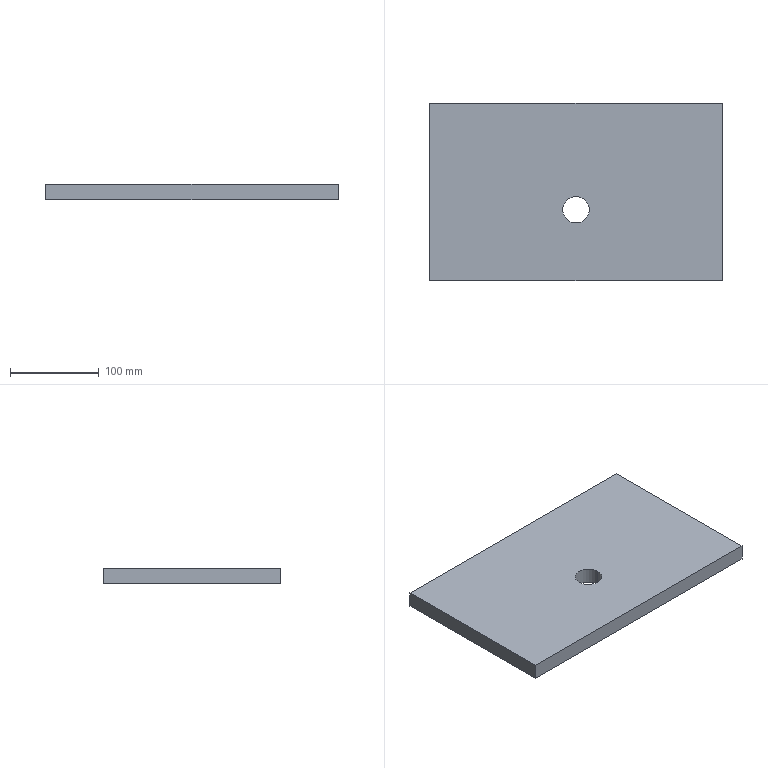Part | STEP file | PN_0031 | 1 solid | 8 faces | box 330 x 200 x 18 mm | volume 1175277 mm3 | plane 6 | cylinder 2 | commonest cylinder face diameters 30 x2
STEP:
#1=CARTESIAN_POINT('',(0.,0.,0.));
#2=DIRECTION('',(0.,0.,1.));
#3=DIRECTION('',(1.,0.,0.));
#4=AXIS2_PLACEMENT_3D('',#1,#2,#3);
#5=CARTESIAN_POINT('',(-15.,-20.,18.));
#6=VERTEX_POINT('',#5);
#7=CARTESIAN_POINT('',(-15.,-20.,0.));
#8=VERTEX_POINT('',#7);
#9=CARTESIAN_POINT('',(-15.,-20.,18.));
#10=DIRECTION('',(0.,0.,-1.));
#11=VECTOR('',#10,1.);
#12=LINE('',#9,#11);
#13=CARTESIAN_POINT('',(0.,-20.,18.));
#14=DIRECTION('',(0.,0.,-1.));
#15=DIRECTION('',(-1.,0.,0.));
#16=AXIS2_PLACEMENT_3D('',#13,#14,#15);
#17=CYLINDRICAL_SURFACE('',#16,15.);
#18=CARTESIAN_POINT('',(6.283,0.));
#19=DIRECTION('',(0.,1.));
#20=VECTOR('',#19,1.);
#21=LINE('',#18,#20);
#22=(GEOMETRIC_REPRESENTATION_CONTEXT(2)PARAMETRIC_REPRESENTATION_CONTEXT()REPRESENTATION_CONTEXT('',''));
#23=DEFINITIONAL_REPRESENTATION('',(#21),#22);
#24=PCURVE('',#17,#23);
#25=CARTESIAN_POINT('',(0.,-20.,18.));
#26=DIRECTION('',(0.,0.,-1.));
#27=DIRECTION('',(-1.,0.,0.));
#28=AXIS2_PLACEMENT_3D('',#25,#26,#27);
#29=CYLINDRICAL_SURFACE('',#28,15.);
#30=CARTESIAN_POINT('',(0.,0.));
#31=DIRECTION('',(0.,1.));
#32=VECTOR('',#31,1.);
#33=LINE('',#30,#32);
#34=(GEOMETRIC_REPRESENTATION_CONTEXT(2)PARAMETRIC_REPRESENTATION_CONTEXT()REPRESENTATION_CONTEXT('',''));
#35=DEFINITIONAL_REPRESENTATION('',(#33),#34);
#36=PCURVE('',#29,#35);
#37=SURFACE_CURVE('',#12,(#24,#36),.PCURVE_S1.);
#38=EDGE_CURVE('',#6,#8,#37,.T.);
#39=ORIENTED_EDGE('',*,*,#38,.T.);
#40=CARTESIAN_POINT('',(15.,-20.,0.));
#41=VERTEX_POINT('',#40);
#42=CARTESIAN_POINT('',(0.,-20.,0.));
#43=DIRECTION('',(0.,0.,1.));
#44=DIRECTION('',(1.,0.,0.));
#45=AXIS2_PLACEMENT_3D('',#42,#43,#44);
#46=CIRCLE('',#45,15.);
#47=CARTESIAN_POINT('',(9.425,18.));
#48=DIRECTION('',(-1.,0.));
#49=VECTOR('',#48,1.);
#50=LINE('',#47,#49);
#51=(GEOMETRIC_REPRESENTATION_CONTEXT(2)PARAMETRIC_REPRESENTATION_CONTEXT()REPRESENTATION_CONTEXT('',''));
#52=DEFINITIONAL_REPRESENTATION('',(#50),#51);
#53=PCURVE('',#17,#52);
#54=CARTESIAN_POINT('',(165.,-100.,0.));
#55=DIRECTION('',(0.,0.,1.));
#56=DIRECTION('',(1.,0.,0.));
#57=AXIS2_PLACEMENT_3D('',#54,#55,#56);
#58=PLANE('',#57);
#59=CARTESIAN_POINT('',(-165.,80.));
#60=DIRECTION('',(1.,0.));
#61=AXIS2_PLACEMENT_2D('',#59,#60);
#62=CIRCLE('',#61,15.);
#63=(GEOMETRIC_REPRESENTATION_CONTEXT(2)PARAMETRIC_REPRESENTATION_CONTEXT()REPRESENTATION_CONTEXT('',''));
#64=DEFINITIONAL_REPRESENTATION('',(#62),#63);
#65=PCURVE('',#58,#64);
#66=SURFACE_CURVE('',#46,(#53,#65),.PCURVE_S1.);
#67=EDGE_CURVE('',#8,#41,#66,.T.);
#68=ORIENTED_EDGE('',*,*,#67,.T.);
#69=CARTESIAN_POINT('',(15.,-20.,18.));
#70=VERTEX_POINT('',#69);
#71=CARTESIAN_POINT('',(15.,-20.,18.));
#72=DIRECTION('',(0.,0.,-1.));
#73=VECTOR('',#72,1.);
#74=LINE('',#71,#73);
#75=CARTESIAN_POINT('',(3.142,0.));
#76=DIRECTION('',(0.,1.));
#77=VECTOR('',#76,1.);
#78=LINE('',#75,#77);
#79=(GEOMETRIC_REPRESENTATION_CONTEXT(2)PARAMETRIC_REPRESENTATION_CONTEXT()REPRESENTATION_CONTEXT('',''));
#80=DEFINITIONAL_REPRESENTATION('',(#78),#79);
#81=PCURVE('',#17,#80);
#82=CARTESIAN_POINT('',(3.142,0.));
#83=DIRECTION('',(0.,1.));
#84=VECTOR('',#83,1.);
#85=LINE('',#82,#84);
#86=(GEOMETRIC_REPRESENTATION_CONTEXT(2)PARAMETRIC_REPRESENTATION_CONTEXT()REPRESENTATION_CONTEXT('',''));
#87=DEFINITIONAL_REPRESENTATION('',(#85),#86);
#88=PCURVE('',#29,#87);
#89=SURFACE_CURVE('',#74,(#81,#88),.PCURVE_S1.);
#90=EDGE_CURVE('',#70,#41,#89,.T.);
#91=ORIENTED_EDGE('',*,*,#90,.F.);
#92=CARTESIAN_POINT('',(0.,-20.,18.));
#93=DIRECTION('',(0.,0.,1.));
#94=DIRECTION('',(1.,0.,0.));
#95=AXIS2_PLACEMENT_3D('',#92,#93,#94);
#96=CIRCLE('',#95,15.);
#97=CARTESIAN_POINT('',(9.425,0.));
#98=DIRECTION('',(-1.,0.));
#99=VECTOR('',#98,1.);
#100=LINE('',#97,#99);
#101=(GEOMETRIC_REPRESENTATION_CONTEXT(2)PARAMETRIC_REPRESENTATION_CONTEXT()REPRESENTATION_CONTEXT('',''));
#102=DEFINITIONAL_REPRESENTATION('',(#100),#101);
#103=PCURVE('',#17,#102);
#104=CARTESIAN_POINT('',(165.,-100.,18.));
#105=DIRECTION('',(0.,0.,1.));
#106=DIRECTION('',(1.,0.,0.));
#107=AXIS2_PLACEMENT_3D('',#104,#105,#106);
#108=PLANE('',#107);
#109=CARTESIAN_POINT('',(-165.,80.));
#110=DIRECTION('',(1.,0.));
#111=AXIS2_PLACEMENT_2D('',#109,#110);
#112=CIRCLE('',#111,15.);
#113=(GEOMETRIC_REPRESENTATION_CONTEXT(2)PARAMETRIC_REPRESENTATION_CONTEXT()REPRESENTATION_CONTEXT('',''));
#114=DEFINITIONAL_REPRESENTATION('',(#112),#113);
#115=PCURVE('',#108,#114);
#116=SURFACE_CURVE('',#96,(#103,#115),.PCURVE_S1.);
#117=EDGE_CURVE('',#6,#70,#116,.T.);
#118=ORIENTED_EDGE('',*,*,#117,.F.);
#119=EDGE_LOOP('',(#39,#68,#91,#118));
#120=FACE_BOUND('',#119,.F.);
#121=ADVANCED_FACE('',(#120),#17,.F.);
#122=CARTESIAN_POINT('',(165.,-100.,18.));
#123=VERTEX_POINT('',#122);
#124=CARTESIAN_POINT('',(165.,100.,18.));
#125=VERTEX_POINT('',#124);
#126=CARTESIAN_POINT('',(165.,100.,18.));
#127=DIRECTION('',(0.,1.,0.));
#128=VECTOR('',#127,1.);
#129=LINE('',#126,#128);
#130=CARTESIAN_POINT('',(0.,200.));
#131=DIRECTION('',(0.,1.));
#132=VECTOR('',#131,1.);
#133=LINE('',#130,#132);
#134=(GEOMETRIC_REPRESENTATION_CONTEXT(2)PARAMETRIC_REPRESENTATION_CONTEXT()REPRESENTATION_CONTEXT('',''));
#135=DEFINITIONAL_REPRESENTATION('',(#133),#134);
#136=PCURVE('',#108,#135);
#137=CARTESIAN_POINT('',(165.,100.,18.));
#138=DIRECTION('',(-1.,0.,0.));
#139=DIRECTION('',(0.,0.,1.));
#140=AXIS2_PLACEMENT_3D('',#137,#138,#139);
#141=PLANE('',#140);
#142=CARTESIAN_POINT('',(0.,0.));
#143=DIRECTION('',(0.,1.));
#144=VECTOR('',#143,1.);
#145=LINE('',#142,#144);
#146=(GEOMETRIC_REPRESENTATION_CONTEXT(2)PARAMETRIC_REPRESENTATION_CONTEXT()REPRESENTATION_CONTEXT('',''));
#147=DEFINITIONAL_REPRESENTATION('',(#145),#146);
#148=PCURVE('',#141,#147);
#149=SURFACE_CURVE('',#129,(#136,#148),.PCURVE_S1.);
#150=EDGE_CURVE('',#123,#125,#149,.T.);
#151=ORIENTED_EDGE('',*,*,#150,.T.);
#152=CARTESIAN_POINT('',(-165.,100.,18.));
#153=VERTEX_POINT('',#152);
#154=CARTESIAN_POINT('',(-165.,100.,18.));
#155=DIRECTION('',(-1.,0.,0.));
#156=VECTOR('',#155,1.);
#157=LINE('',#154,#156);
#158=CARTESIAN_POINT('',(-330.,200.));
#159=DIRECTION('',(-1.,0.));
#160=VECTOR('',#159,1.);
#161=LINE('',#158,#160);
#162=(GEOMETRIC_REPRESENTATION_CONTEXT(2)PARAMETRIC_REPRESENTATION_CONTEXT()REPRESENTATION_CONTEXT('',''));
#163=DEFINITIONAL_REPRESENTATION('',(#161),#162);
#164=PCURVE('',#108,#163);
#165=CARTESIAN_POINT('',(-165.,100.,18.));
#166=DIRECTION('',(0.,-1.,0.));
#167=DIRECTION('',(0.,0.,-1.));
#168=AXIS2_PLACEMENT_3D('',#165,#166,#167);
#169=PLANE('',#168);
#170=CARTESIAN_POINT('',(0.,0.));
#171=DIRECTION('',(0.,-1.));
#172=VECTOR('',#171,1.);
#173=LINE('',#170,#172);
#174=(GEOMETRIC_REPRESENTATION_CONTEXT(2)PARAMETRIC_REPRESENTATION_CONTEXT()REPRESENTATION_CONTEXT('',''));
#175=DEFINITIONAL_REPRESENTATION('',(#173),#174);
#176=PCURVE('',#169,#175);
#177=SURFACE_CURVE('',#157,(#164,#176),.PCURVE_S1.);
#178=EDGE_CURVE('',#125,#153,#177,.T.);
#179=ORIENTED_EDGE('',*,*,#178,.T.);
#180=CARTESIAN_POINT('',(-165.,-100.,18.));
#181=VERTEX_POINT('',#180);
#182=CARTESIAN_POINT('',(-165.,100.,18.));
#183=DIRECTION('',(0.,-1.,0.));
#184=VECTOR('',#183,1.);
#185=LINE('',#182,#184);
#186=CARTESIAN_POINT('',(-330.,200.));
#187=DIRECTION('',(0.,-1.));
#188=VECTOR('',#187,1.);
#189=LINE('',#186,#188);
#190=(GEOMETRIC_REPRESENTATION_CONTEXT(2)PARAMETRIC_REPRESENTATION_CONTEXT()REPRESENTATION_CONTEXT('',''));
#191=DEFINITIONAL_REPRESENTATION('',(#189),#190);
#192=PCURVE('',#108,#191);
#193=CARTESIAN_POINT('',(-165.,100.,18.));
#194=DIRECTION('',(1.,0.,0.));
#195=DIRECTION('',(0.,1.,0.));
#196=AXIS2_PLACEMENT_3D('',#193,#194,#195);
#197=PLANE('',#196);
#198=CARTESIAN_POINT('',(0.,0.));
#199=DIRECTION('',(-1.,0.));
#200=VECTOR('',#199,1.);
#201=LINE('',#198,#200);
#202=(GEOMETRIC_REPRESENTATION_CONTEXT(2)PARAMETRIC_REPRESENTATION_CONTEXT()REPRESENTATION_CONTEXT('',''));
#203=DEFINITIONAL_REPRESENTATION('',(#201),#202);
#204=PCURVE('',#197,#203);
#205=SURFACE_CURVE('',#185,(#192,#204),.PCURVE_S1.);
#206=EDGE_CURVE('',#153,#181,#205,.T.);
#207=ORIENTED_EDGE('',*,*,#206,.T.);
#208=CARTESIAN_POINT('',(-165.,-100.,18.));
#209=DIRECTION('',(1.,0.,0.));
#210=VECTOR('',#209,1.);
#211=LINE('',#208,#210);
#212=CARTESIAN_POINT('',(-330.,0.));
#213=DIRECTION('',(1.,0.));
#214=VECTOR('',#213,1.);
#215=LINE('',#212,#214);
#216=(GEOMETRIC_REPRESENTATION_CONTEXT(2)PARAMETRIC_REPRESENTATION_CONTEXT()REPRESENTATION_CONTEXT('',''));
#217=DEFINITIONAL_REPRESENTATION('',(#215),#216);
#218=PCURVE('',#108,#217);
#219=CARTESIAN_POINT('',(-165.,-100.,18.));
#220=DIRECTION('',(0.,1.,0.));
#221=DIRECTION('',(-1.,0.,0.));
#222=AXIS2_PLACEMENT_3D('',#219,#220,#221);
#223=PLANE('',#222);
#224=CARTESIAN_POINT('',(0.,0.));
#225=DIRECTION('',(-1.,0.));
#226=VECTOR('',#225,1.);
#227=LINE('',#224,#226);
#228=(GEOMETRIC_REPRESENTATION_CONTEXT(2)PARAMETRIC_REPRESENTATION_CONTEXT()REPRESENTATION_CONTEXT('',''));
#229=DEFINITIONAL_REPRESENTATION('',(#227),#228);
#230=PCURVE('',#223,#229);
#231=SURFACE_CURVE('',#211,(#218,#230),.PCURVE_S1.);
#232=EDGE_CURVE('',#181,#123,#231,.T.);
#233=ORIENTED_EDGE('',*,*,#232,.T.);
#234=EDGE_LOOP('',(#151,#179,#207,#233));
#235=FACE_BOUND('',#234,.T.);
#236=ORIENTED_EDGE('',*,*,#117,.F.);
#237=CARTESIAN_POINT('',(0.,-20.,18.));
#238=DIRECTION('',(0.,0.,1.));
#239=DIRECTION('',(1.,0.,0.));
#240=AXIS2_PLACEMENT_3D('',#237,#238,#239);
#241=CIRCLE('',#240,15.);
#242=CARTESIAN_POINT('',(-165.,80.));
#243=DIRECTION('',(1.,0.));
#244=AXIS2_PLACEMENT_2D('',#242,#243);
#245=CIRCLE('',#244,15.);
#246=(GEOMETRIC_REPRESENTATION_CONTEXT(2)PARAMETRIC_REPRESENTATION_CONTEXT()REPRESENTATION_CONTEXT('',''));
#247=DEFINITIONAL_REPRESENTATION('',(#245),#246);
#248=PCURVE('',#108,#247);
#249=CARTESIAN_POINT('',(3.142,0.));
#250=DIRECTION('',(-1.,0.));
#251=VECTOR('',#250,1.);
#252=LINE('',#249,#251);
#253=(GEOMETRIC_REPRESENTATION_CONTEXT(2)PARAMETRIC_REPRESENTATION_CONTEXT()REPRESENTATION_CONTEXT('',''));
#254=DEFINITIONAL_REPRESENTATION('',(#252),#253);
#255=PCURVE('',#29,#254);
#256=SURFACE_CURVE('',#241,(#248,#255),.PCURVE_S1.);
#257=EDGE_CURVE('',#70,#6,#256,.T.);
#258=ORIENTED_EDGE('',*,*,#257,.F.);
#259=EDGE_LOOP('',(#236,#258));
#260=FACE_BOUND('',#259,.T.);
#261=ADVANCED_FACE('',(#235,#260),#108,.T.);
#262=CARTESIAN_POINT('',(165.,-100.,0.));
#263=VERTEX_POINT('',#262);
#264=CARTESIAN_POINT('',(165.,100.,0.));
#265=VERTEX_POINT('',#264);
#266=CARTESIAN_POINT('',(165.,100.,0.));
#267=DIRECTION('',(0.,1.,0.));
#268=VECTOR('',#267,1.);
#269=LINE('',#266,#268);
#270=CARTESIAN_POINT('',(0.,200.));
#271=DIRECTION('',(0.,1.));
#272=VECTOR('',#271,1.);
#273=LINE('',#270,#272);
#274=(GEOMETRIC_REPRESENTATION_CONTEXT(2)PARAMETRIC_REPRESENTATION_CONTEXT()REPRESENTATION_CONTEXT('',''));
#275=DEFINITIONAL_REPRESENTATION('',(#273),#274);
#276=PCURVE('',#58,#275);
#277=CARTESIAN_POINT('',(-18.,0.));
#278=DIRECTION('',(0.,1.));
#279=VECTOR('',#278,1.);
#280=LINE('',#277,#279);
#281=(GEOMETRIC_REPRESENTATION_CONTEXT(2)PARAMETRIC_REPRESENTATION_CONTEXT()REPRESENTATION_CONTEXT('',''));
#282=DEFINITIONAL_REPRESENTATION('',(#280),#281);
#283=PCURVE('',#141,#282);
#284=SURFACE_CURVE('',#269,(#276,#283),.PCURVE_S1.);
#285=EDGE_CURVE('',#263,#265,#284,.T.);
#286=ORIENTED_EDGE('',*,*,#285,.F.);
#287=CARTESIAN_POINT('',(-165.,-100.,0.));
#288=VERTEX_POINT('',#287);
#289=CARTESIAN_POINT('',(-165.,-100.,0.));
#290=DIRECTION('',(1.,0.,0.));
#291=VECTOR('',#290,1.);
#292=LINE('',#289,#291);
#293=CARTESIAN_POINT('',(-330.,0.));
#294=DIRECTION('',(1.,0.));
#295=VECTOR('',#294,1.);
#296=LINE('',#293,#295);
#297=(GEOMETRIC_REPRESENTATION_CONTEXT(2)PARAMETRIC_REPRESENTATION_CONTEXT()REPRESENTATION_CONTEXT('',''));
#298=DEFINITIONAL_REPRESENTATION('',(#296),#297);
#299=PCURVE('',#58,#298);
#300=CARTESIAN_POINT('',(0.,-18.));
#301=DIRECTION('',(-1.,0.));
#302=VECTOR('',#301,1.);
#303=LINE('',#300,#302);
#304=(GEOMETRIC_REPRESENTATION_CONTEXT(2)PARAMETRIC_REPRESENTATION_CONTEXT()REPRESENTATION_CONTEXT('',''));
#305=DEFINITIONAL_REPRESENTATION('',(#303),#304);
#306=PCURVE('',#223,#305);
#307=SURFACE_CURVE('',#292,(#299,#306),.PCURVE_S1.);
#308=EDGE_CURVE('',#288,#263,#307,.T.);
#309=ORIENTED_EDGE('',*,*,#308,.F.);
#310=CARTESIAN_POINT('',(-165.,100.,0.));
#311=VERTEX_POINT('',#310);
#312=CARTESIAN_POINT('',(-165.,100.,0.));
#313=DIRECTION('',(0.,-1.,0.));
#314=VECTOR('',#313,1.);
#315=LINE('',#312,#314);
#316=CARTESIAN_POINT('',(-330.,200.));
#317=DIRECTION('',(0.,-1.));
#318=VECTOR('',#317,1.);
#319=LINE('',#316,#318);
#320=(GEOMETRIC_REPRESENTATION_CONTEXT(2)PARAMETRIC_REPRESENTATION_CONTEXT()REPRESENTATION_CONTEXT('',''));
#321=DEFINITIONAL_REPRESENTATION('',(#319),#320);
#322=PCURVE('',#58,#321);
#323=CARTESIAN_POINT('',(0.,-18.));
#324=DIRECTION('',(-1.,0.));
#325=VECTOR('',#324,1.);
#326=LINE('',#323,#325);
#327=(GEOMETRIC_REPRESENTATION_CONTEXT(2)PARAMETRIC_REPRESENTATION_CONTEXT()REPRESENTATION_CONTEXT('',''));
#328=DEFINITIONAL_REPRESENTATION('',(#326),#327);
#329=PCURVE('',#197,#328);
#330=SURFACE_CURVE('',#315,(#322,#329),.PCURVE_S1.);
#331=EDGE_CURVE('',#311,#288,#330,.T.);
#332=ORIENTED_EDGE('',*,*,#331,.F.);
#333=CARTESIAN_POINT('',(-165.,100.,0.));
#334=DIRECTION('',(-1.,0.,0.));
#335=VECTOR('',#334,1.);
#336=LINE('',#333,#335);
#337=CARTESIAN_POINT('',(-330.,200.));
#338=DIRECTION('',(-1.,0.));
#339=VECTOR('',#338,1.);
#340=LINE('',#337,#339);
#341=(GEOMETRIC_REPRESENTATION_CONTEXT(2)PARAMETRIC_REPRESENTATION_CONTEXT()REPRESENTATION_CONTEXT('',''));
#342=DEFINITIONAL_REPRESENTATION('',(#340),#341);
#343=PCURVE('',#58,#342);
#344=CARTESIAN_POINT('',(18.,0.));
#345=DIRECTION('',(0.,-1.));
#346=VECTOR('',#345,1.);
#347=LINE('',#344,#346);
#348=(GEOMETRIC_REPRESENTATION_CONTEXT(2)PARAMETRIC_REPRESENTATION_CONTEXT()REPRESENTATION_CONTEXT('',''));
#349=DEFINITIONAL_REPRESENTATION('',(#347),#348);
#350=PCURVE('',#169,#349);
#351=SURFACE_CURVE('',#336,(#343,#350),.PCURVE_S1.);
#352=EDGE_CURVE('',#265,#311,#351,.T.);
#353=ORIENTED_EDGE('',*,*,#352,.F.);
#354=EDGE_LOOP('',(#286,#309,#332,#353));
#355=FACE_BOUND('',#354,.T.);
#356=ORIENTED_EDGE('',*,*,#67,.T.);
#357=CARTESIAN_POINT('',(0.,-20.,0.));
#358=DIRECTION('',(0.,0.,1.));
#359=DIRECTION('',(1.,0.,0.));
#360=AXIS2_PLACEMENT_3D('',#357,#358,#359);
#361=CIRCLE('',#360,15.);
#362=CARTESIAN_POINT('',(-165.,80.));
#363=DIRECTION('',(1.,0.));
#364=AXIS2_PLACEMENT_2D('',#362,#363);
#365=CIRCLE('',#364,15.);
#366=(GEOMETRIC_REPRESENTATION_CONTEXT(2)PARAMETRIC_REPRESENTATION_CONTEXT()REPRESENTATION_CONTEXT('',''));
#367=DEFINITIONAL_REPRESENTATION('',(#365),#366);
#368=PCURVE('',#58,#367);
#369=CARTESIAN_POINT('',(3.142,18.));
#370=DIRECTION('',(-1.,0.));
#371=VECTOR('',#370,1.);
#372=LINE('',#369,#371);
#373=(GEOMETRIC_REPRESENTATION_CONTEXT(2)PARAMETRIC_REPRESENTATION_CONTEXT()REPRESENTATION_CONTEXT('',''));
#374=DEFINITIONAL_REPRESENTATION('',(#372),#373);
#375=PCURVE('',#29,#374);
#376=SURFACE_CURVE('',#361,(#368,#375),.PCURVE_S1.);
#377=EDGE_CURVE('',#41,#8,#376,.T.);
#378=ORIENTED_EDGE('',*,*,#377,.T.);
#379=EDGE_LOOP('',(#356,#378));
#380=FACE_BOUND('',#379,.T.);
#381=ADVANCED_FACE('',(#355,#380),#58,.F.);
#382=ORIENTED_EDGE('',*,*,#285,.T.);
#383=CARTESIAN_POINT('',(165.,100.,18.));
#384=DIRECTION('',(0.,0.,-1.));
#385=VECTOR('',#384,1.);
#386=LINE('',#383,#385);
#387=CARTESIAN_POINT('',(0.,0.));
#388=DIRECTION('',(-1.,0.));
#389=VECTOR('',#388,1.);
#390=LINE('',#387,#389);
#391=(GEOMETRIC_REPRESENTATION_CONTEXT(2)PARAMETRIC_REPRESENTATION_CONTEXT()REPRESENTATION_CONTEXT('',''));
#392=DEFINITIONAL_REPRESENTATION('',(#390),#391);
#393=PCURVE('',#141,#392);
#394=CARTESIAN_POINT('',(0.,330.));
#395=DIRECTION('',(1.,0.));
#396=VECTOR('',#395,1.);
#397=LINE('',#394,#396);
#398=(GEOMETRIC_REPRESENTATION_CONTEXT(2)PARAMETRIC_REPRESENTATION_CONTEXT()REPRESENTATION_CONTEXT('',''));
#399=DEFINITIONAL_REPRESENTATION('',(#397),#398);
#400=PCURVE('',#169,#399);
#401=SURFACE_CURVE('',#386,(#393,#400),.PCURVE_S1.);
#402=EDGE_CURVE('',#125,#265,#401,.T.);
#403=ORIENTED_EDGE('',*,*,#402,.F.);
#404=ORIENTED_EDGE('',*,*,#150,.F.);
#405=CARTESIAN_POINT('',(165.,-100.,18.));
#406=DIRECTION('',(0.,0.,-1.));
#407=VECTOR('',#406,1.);
#408=LINE('',#405,#407);
#409=CARTESIAN_POINT('',(0.,-200.));
#410=DIRECTION('',(-1.,0.));
#411=VECTOR('',#410,1.);
#412=LINE('',#409,#411);
#413=(GEOMETRIC_REPRESENTATION_CONTEXT(2)PARAMETRIC_REPRESENTATION_CONTEXT()REPRESENTATION_CONTEXT('',''));
#414=DEFINITIONAL_REPRESENTATION('',(#412),#413);
#415=PCURVE('',#141,#414);
#416=CARTESIAN_POINT('',(-330.,0.));
#417=DIRECTION('',(0.,-1.));
#418=VECTOR('',#417,1.);
#419=LINE('',#416,#418);
#420=(GEOMETRIC_REPRESENTATION_CONTEXT(2)PARAMETRIC_REPRESENTATION_CONTEXT()REPRESENTATION_CONTEXT('',''));
#421=DEFINITIONAL_REPRESENTATION('',(#419),#420);
#422=PCURVE('',#223,#421);
#423=SURFACE_CURVE('',#408,(#415,#422),.PCURVE_S1.);
#424=EDGE_CURVE('',#123,#263,#423,.T.);
#425=ORIENTED_EDGE('',*,*,#424,.T.);
#426=EDGE_LOOP('',(#382,#403,#404,#425));
#427=FACE_BOUND('',#426,.T.);
#428=ADVANCED_FACE('',(#427),#141,.F.);
#429=ORIENTED_EDGE('',*,*,#352,.T.);
#430=CARTESIAN_POINT('',(-165.,100.,18.));
#431=DIRECTION('',(0.,0.,-1.));
#432=VECTOR('',#431,1.);
#433=LINE('',#430,#432);
#434=CARTESIAN_POINT('',(0.,0.));
#435=DIRECTION('',(1.,0.));
#436=VECTOR('',#435,1.);
#437=LINE('',#434,#436);
#438=(GEOMETRIC_REPRESENTATION_CONTEXT(2)PARAMETRIC_REPRESENTATION_CONTEXT()REPRESENTATION_CONTEXT('',''));
#439=DEFINITIONAL_REPRESENTATION('',(#437),#438);
#440=PCURVE('',#169,#439);
#441=CARTESIAN_POINT('',(0.,0.));
#442=DIRECTION('',(0.,-1.));
#443=VECTOR('',#442,1.);
#444=LINE('',#441,#443);
#445=(GEOMETRIC_REPRESENTATION_CONTEXT(2)PARAMETRIC_REPRESENTATION_CONTEXT()REPRESENTATION_CONTEXT('',''));
#446=DEFINITIONAL_REPRESENTATION('',(#444),#445);
#447=PCURVE('',#197,#446);
#448=SURFACE_CURVE('',#433,(#440,#447),.PCURVE_S1.);
#449=EDGE_CURVE('',#153,#311,#448,.T.);
#450=ORIENTED_EDGE('',*,*,#449,.F.);
#451=ORIENTED_EDGE('',*,*,#178,.F.);
#452=ORIENTED_EDGE('',*,*,#402,.T.);
#453=EDGE_LOOP('',(#429,#450,#451,#452));
#454=FACE_BOUND('',#453,.T.);
#455=ADVANCED_FACE('',(#454),#169,.F.);
#456=ORIENTED_EDGE('',*,*,#331,.T.);
#457=CARTESIAN_POINT('',(-165.,-100.,18.));
#458=DIRECTION('',(0.,0.,-1.));
#459=VECTOR('',#458,1.);
#460=LINE('',#457,#459);
#461=CARTESIAN_POINT('',(-200.,0.));
#462=DIRECTION('',(0.,-1.));
#463=VECTOR('',#462,1.);
#464=LINE('',#461,#463);
#465=(GEOMETRIC_REPRESENTATION_CONTEXT(2)PARAMETRIC_REPRESENTATION_CONTEXT()REPRESENTATION_CONTEXT('',''));
#466=DEFINITIONAL_REPRESENTATION('',(#464),#465);
#467=PCURVE('',#197,#466);
#468=CARTESIAN_POINT('',(0.,0.));
#469=DIRECTION('',(0.,-1.));
#470=VECTOR('',#469,1.);
#471=LINE('',#468,#470);
#472=(GEOMETRIC_REPRESENTATION_CONTEXT(2)PARAMETRIC_REPRESENTATION_CONTEXT()REPRESENTATION_CONTEXT('',''));
#473=DEFINITIONAL_REPRESENTATION('',(#471),#472);
#474=PCURVE('',#223,#473);
#475=SURFACE_CURVE('',#460,(#467,#474),.PCURVE_S1.);
#476=EDGE_CURVE('',#181,#288,#475,.T.);
#477=ORIENTED_EDGE('',*,*,#476,.F.);
#478=ORIENTED_EDGE('',*,*,#206,.F.);
#479=ORIENTED_EDGE('',*,*,#449,.T.);
#480=EDGE_LOOP('',(#456,#477,#478,#479));
#481=FACE_BOUND('',#480,.T.);
#482=ADVANCED_FACE('',(#481),#197,.F.);
#483=ORIENTED_EDGE('',*,*,#308,.T.);
#484=ORIENTED_EDGE('',*,*,#424,.F.);
#485=ORIENTED_EDGE('',*,*,#232,.F.);
#486=ORIENTED_EDGE('',*,*,#476,.T.);
#487=EDGE_LOOP('',(#483,#484,#485,#486));
#488=FACE_BOUND('',#487,.T.);
#489=ADVANCED_FACE('',(#488),#223,.F.);
#490=ORIENTED_EDGE('',*,*,#377,.T.);
#491=ORIENTED_EDGE('',*,*,#38,.F.);
#492=ORIENTED_EDGE('',*,*,#257,.F.);
#493=ORIENTED_EDGE('',*,*,#90,.T.);
#494=EDGE_LOOP('',(#490,#491,#492,#493));
#495=FACE_BOUND('',#494,.F.);
#496=ADVANCED_FACE('',(#495),#29,.F.);
#497=CLOSED_SHELL('',(#121,#261,#381,#428,#455,#482,#489,#496));
#498=MANIFOLD_SOLID_BREP('',#497);
#499=(LENGTH_UNIT()NAMED_UNIT(*)SI_UNIT(.MILLI.,.METRE.));
#500=UNCERTAINTY_MEASURE_WITH_UNIT(LENGTH_MEASURE(0.0000001),#499,'','');
#501=(NAMED_UNIT(*)PLANE_ANGLE_UNIT()SI_UNIT($,.RADIAN.));
#502=(NAMED_UNIT(*)SI_UNIT($,.STERADIAN.)SOLID_ANGLE_UNIT());
#503=(GEOMETRIC_REPRESENTATION_CONTEXT(3)GLOBAL_UNCERTAINTY_ASSIGNED_CONTEXT((#500))GLOBAL_UNIT_ASSIGNED_CONTEXT((#499,#501,#502))REPRESENTATION_CONTEXT('',''));
#504=ADVANCED_BREP_SHAPE_REPRESENTATION('',(#4,#498),#503);